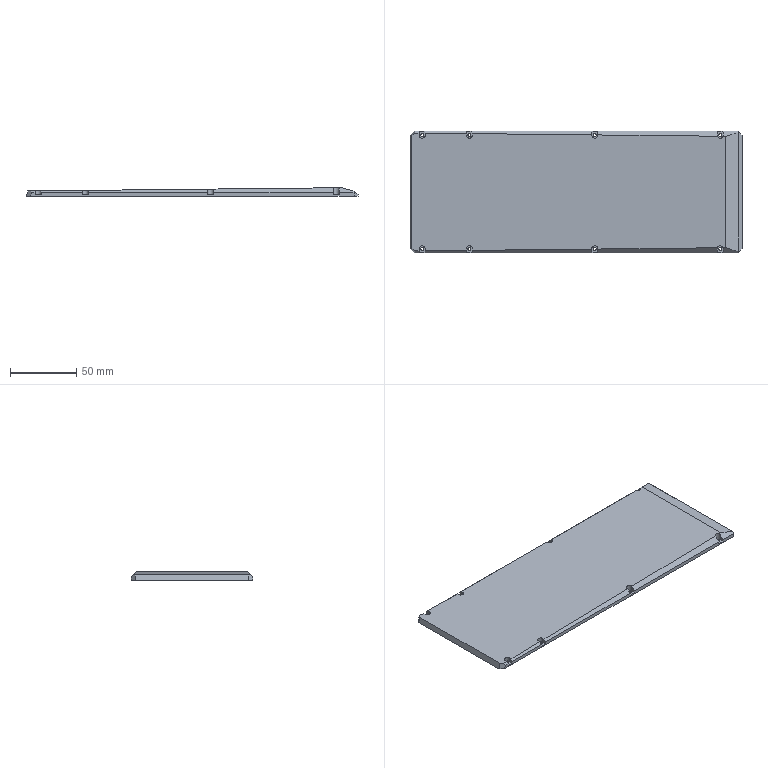NC program | NX | posted with a generic post | part box 251.5 x 92 x 6.5 mm
Whole program:
N10 G17 G21 G94 G90
(PLANAR_MILL_COPY_COPY , TOOL : D6-18-D6-50-3T-FINISH)
N12 T03 M6
N14 G53
N16 G17 G0 G90 X37.394 Y-34.9 S4000 M3
N18 G43 Z30. H3
N20 Z-1.2
N22 G94 G1 Z-3.2 F800.
N24 G3 X39.394 Y-36.9 R2.
N26 G1 X42.9
N28 Y-33.394
N30 G3 X40.9 Y-31.394 R2.
N32 G1 Z-1.2
N34 G0 Z30.
N36 Y31.394
N38 Z-1.2
N40 G1 Z-3.2
N42 G3 X42.9 Y33.394 R2.
N44 G1 Y36.9
N46 X39.394
N48 G3 X37.394 Y34.9 R2.
N50 G1 Z-1.2
N52 G0 Z30.
N54 X-95.394
N56 Z-1.2
N58 G1 Z-3.2
N60 G3 X-97.394 Y36.9 R2.
N62 G1 X-100.9
N64 Y33.394
N66 G3 X-98.9 Y31.394 R2.
N68 G1 Z-1.2
N70 G0 Z30.
N72 Y-31.394
N74 Z-1.2
N76 G1 Z-3.2
N78 G3 X-100.9 Y-33.394 R2.
N80 G1 Y-36.9
N82 X-97.394
N84 G3 X-95.394 Y-34.9 R2.
N86 G1 Z-1.2
N88 G0 Z30.
(PLANAR_MILL_COPY_COPY_COPY_1 , TOOL : D6-18-D6-50-3T-FINISH)
N90 X102.394
N92 Z0.3
N94 G1 Z-1.7
N96 G3 X104.394 Y-36.9 R2.
N98 G1 X107.9
N100 Y-33.394
N102 G3 X105.9 Y-31.394 R2.
N104 G1 Z0.3
N106 G0 Z30.
N108 Y31.394
N110 Z0.3
N112 G1 Z-1.7
N114 G3 X107.9 Y33.394 R2.
N116 G1 Y36.9
N118 X104.394
N120 G3 X102.394 Y34.9 R2.
N122 G1 Z0.3
N124 G0 Z30.
(PLANAR_MILL_COPY , TOOL : D6-18-D6-50-3T-FINISH)
N126 X40. Y0.
N128 Z1.3
N130 G1 Z-1.7
N132 X46.
N134 Y36.9
N136 X107.9
N138 Y-36.9
N140 X46.
N142 Y0.
N144 X50.8
N146 Y32.1
N148 X103.1
N150 Y-32.1
N152 X50.8
N154 Y0.
N156 X55.6
N158 Y27.3
N160 X98.3
N162 Y-27.3
N164 X55.6
N166 Y0.
N168 X60.4
N170 Y22.5
N172 X93.5
N174 Y-22.5
N176 X60.4
N178 Y0.
N180 X65.2
N182 Y17.7
N184 X88.7
N186 Y-17.7
N188 X65.2
N190 Y0.
N192 X70.
N194 Y12.9
N196 X83.9
N198 Y-12.9
N200 X70.
N202 Y0.
N204 X74.8
N206 Y8.1
N208 X79.1
N210 Y-8.1
N212 X74.8
N214 Y0.
N216 X71.8
N218 Z1.3
N220 G0 Z30.
(PLANAR_MILL_COPY_COPY_1 , TOOL : D6-18-D6-50-3T-FINISH)
N222 X-31.498 Y-3.425
N224 Z-2.2
N226 G3 X-31.498 Y-3.425 Z-2.792 I2.498 J1.025
N228 X-29. Y0.3 Z-3.2 R-2.7
N230 G1 X-64.3
N232 Y-0.3
N234 X6.3
N236 Y0.3
N238 X-29.
N240 Y3.3
N242 X-67.3
N244 Y-3.3
N246 X9.3
N248 Y3.3
N250 X-29.
N252 Y8.1
N254 X-72.1
N256 Y-8.1
N258 X14.1
N260 Y8.1
N262 X-29.
N264 Y12.9
N266 X-76.9
N268 Y-12.9
N270 X18.9
N272 Y12.9
N274 X-29.
N276 Y17.7
N278 X-81.7
N280 Y-17.7
N282 X23.7
N284 Y17.7
N286 X-29.
N288 Y22.5
N290 X-86.5
N292 Y-22.5
N294 X28.5
N296 Y22.5
N298 X-29.
N300 Y27.3
N302 X-91.3
N304 Y-27.3
N306 X33.3
N308 Y27.3
N310 X-29.
N312 Y32.1
N314 X-96.1
N316 Y-32.1
N318 X38.1
N320 Y32.1
N322 X-29.
N324 Y36.9
N326 X-100.9
N328 Y-36.9
N330 X42.9
N332 Y36.9
N334 X-29.
N336 Y33.9
N338 Z-0.2
N340 G0 Z30.
(PLANAR_MILL_5_COPY , TOOL : D6-18-D6-50-3T-FINISH)
N342 X-64.7 Y28.31 S6500
N344 Z-3.8
N346 G1 Y29.8 Z-3.826
N348 X-70.3 Z-3.924
N350 Y14.2 Z-4.196
N352 X-64.7 Z-4.294
N354 Y29.8 Z-4.566
N356 X-70.3 Z-4.664
N358 Y22. Z-4.8
N360 Y14.2
N362 X-64.7
N364 Y29.8
N366 X-70.3
N368 Y22.
N370 X-74.5
N372 Y10.
N374 X-60.5
N376 Y34.
N378 X-74.5
N380 Y22.
N382 X-71.5
N384 Z-1.8
N386 G0 Z30.
N388 M5
(平面铣倒角 , TOOL : CHAMFERD4-90DEG)
N390 T04 M6
N392 G53
N394 G17 G0 G90 X4.119 Y38.836 S3500 M3
N396 G43 Z30. H4
N398 Z2.
N400 G94 G1 Z-1. F1000.
N402 G41 X3.64 Y38.98 D4
N404 X3.5 Y39.
N406 X-101.
N408 G3 X-103. Y37. R2.
N410 G1 Y-37.
N412 G3 X-101. Y-39. R2.
N414 G1 X108.
N416 G3 X110. Y-37. R2.
N418 G1 Y37.
N420 G3 X108. Y39. R2.
N422 G1 X3.5
N424 X3.36 Y38.98
N426 G40
N428 X2.881 Y38.836
N430 Z2.
N432 G0 Z30.
(PLANAR_MILL_5_COPY_COPY , TOOL : CHAMFERD4-90DEG)
N434 X-75.6 Y23. S4500
N436 Z-2.6
N438 G1 Z-4.6 F600.
N440 G3 X-76.6 Y22. R1.
N442 G1 Y10.
N444 G3 X-74.5 Y7.9 R2.1
N446 G1 X-60.5
N448 G3 X-58.4 Y10. R2.1
N450 G1 Y34.
N452 G3 X-60.5 Y36.1 R2.1
N454 G1 X-74.5
N456 G3 X-76.6 Y34. R2.1
N458 G1 Y22.
N460 G3 X-75.6 Y21. R1.
N462 G1 X-76.1 Y23.
N464 G3 X-77.1 Y22. R1.
N466 G1 Y10.
N468 G3 X-74.5 Y7.4 R2.6
N470 G1 X-60.5
N472 G3 X-57.9 Y10. R2.6
N474 G1 Y34.
N476 G3 X-60.5 Y36.6 R2.6
N478 G1 X-74.5
N480 G3 X-77.1 Y34. R2.6
N482 G1 Y22.
N484 G3 X-76.1 Y21. R1.
N486 G1 Z-2.6
N488 G0 Z30.
N490 M5
N492 M2